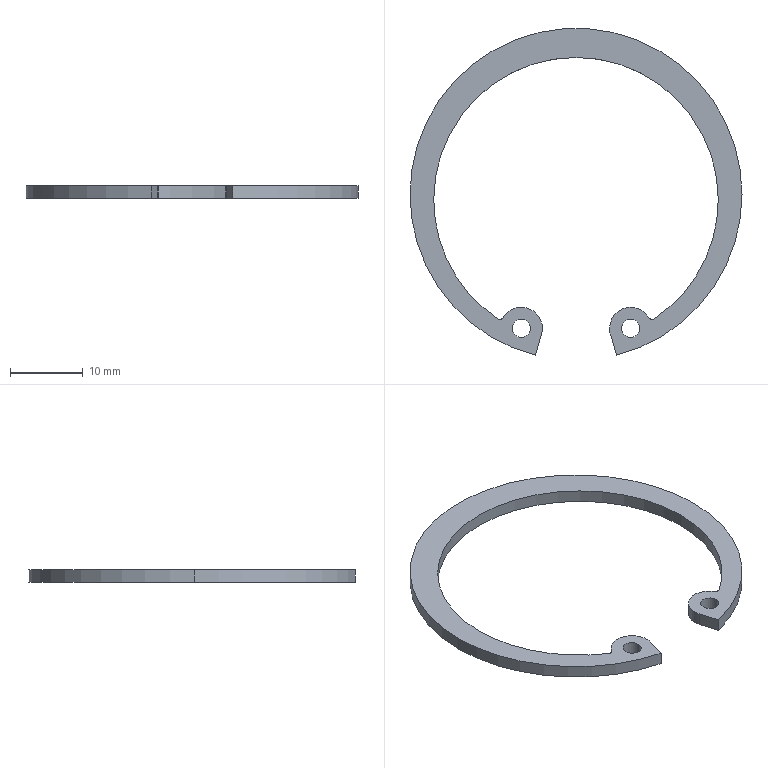Part | STEP file | BFU-2-42(2)^BFU71-6004ZZ-L55-S20_Drive roller assembly | 1 solid | 19 faces | box 45.5 x 44.807 x 1.75 mm | volume 744.242 mm3 | cylinder 15 | plane 4 | commonest cylinder face diameters 2.5 x4 5.8 x3 38.99 x3 45.5 x3 1 x2
STEP:
#1=CARTESIAN_POINT('',(0.,0.,0.));
#2=DIRECTION('',(0.,0.,1.));
#3=DIRECTION('',(1.,0.,0.));
#4=AXIS2_PLACEMENT_3D('',#1,#2,#3);
#5=CARTESIAN_POINT('',(22.75,0.005092,1.75));
#6=VERTEX_POINT('',#5);
#7=CARTESIAN_POINT('',(-22.75,0.005092,1.75));
#8=VERTEX_POINT('',#7);
#9=CARTESIAN_POINT('',(0.,0.005092,1.75));
#10=DIRECTION('',(0.,0.,1.));
#11=DIRECTION('',(1.,0.,0.));
#12=AXIS2_PLACEMENT_3D('',#9,#10,#11);
#13=CIRCLE('',#12,22.75);
#14=CARTESIAN_POINT('',(0.,0.005092,1.75));
#15=DIRECTION('',(0.,0.,-1.));
#16=DIRECTION('',(-1.,0.,0.));
#17=AXIS2_PLACEMENT_3D('',#14,#15,#16);
#18=CYLINDRICAL_SURFACE('',#17,22.75);
#19=CARTESIAN_POINT('',(3.142,0.));
#20=DIRECTION('',(-1.,0.));
#21=VECTOR('',#20,1.);
#22=LINE('',#19,#21);
#23=(GEOMETRIC_REPRESENTATION_CONTEXT(2)PARAMETRIC_REPRESENTATION_CONTEXT()REPRESENTATION_CONTEXT('',''));
#24=DEFINITIONAL_REPRESENTATION('',(#22),#23);
#25=PCURVE('',#18,#24);
#26=CARTESIAN_POINT('',(0.,0.005092,1.75));
#27=DIRECTION('',(0.,0.,1.));
#28=DIRECTION('',(1.,0.,0.));
#29=AXIS2_PLACEMENT_3D('',#26,#27,#28);
#30=PLANE('',#29);
#31=CARTESIAN_POINT('',(0.,0.));
#32=DIRECTION('',(1.,0.));
#33=AXIS2_PLACEMENT_2D('',#31,#32);
#34=CIRCLE('',#33,22.75);
#35=(GEOMETRIC_REPRESENTATION_CONTEXT(2)PARAMETRIC_REPRESENTATION_CONTEXT()REPRESENTATION_CONTEXT('',''));
#36=DEFINITIONAL_REPRESENTATION('',(#34),#35);
#37=PCURVE('',#30,#36);
#38=SURFACE_CURVE('',#13,(#25,#37),.PCURVE_S1.);
#39=EDGE_CURVE('',#6,#8,#38,.T.);
#40=ORIENTED_EDGE('',*,*,#39,.F.);
#41=CARTESIAN_POINT('',(22.75,0.005092,0.));
#42=VERTEX_POINT('',#41);
#43=CARTESIAN_POINT('',(22.75,0.005092,1.75));
#44=DIRECTION('',(0.,0.,-1.));
#45=VECTOR('',#44,1.);
#46=LINE('',#43,#45);
#47=CARTESIAN_POINT('',(3.142,0.));
#48=DIRECTION('',(0.,1.));
#49=VECTOR('',#48,1.);
#50=LINE('',#47,#49);
#51=(GEOMETRIC_REPRESENTATION_CONTEXT(2)PARAMETRIC_REPRESENTATION_CONTEXT()REPRESENTATION_CONTEXT('',''));
#52=DEFINITIONAL_REPRESENTATION('',(#50),#51);
#53=PCURVE('',#18,#52);
#54=CARTESIAN_POINT('',(0.,0.005092,1.75));
#55=DIRECTION('',(0.,0.,-1.));
#56=DIRECTION('',(-1.,0.,0.));
#57=AXIS2_PLACEMENT_3D('',#54,#55,#56);
#58=CYLINDRICAL_SURFACE('',#57,22.75);
#59=CARTESIAN_POINT('',(3.142,0.));
#60=DIRECTION('',(0.,1.));
#61=VECTOR('',#60,1.);
#62=LINE('',#59,#61);
#63=(GEOMETRIC_REPRESENTATION_CONTEXT(2)PARAMETRIC_REPRESENTATION_CONTEXT()REPRESENTATION_CONTEXT('',''));
#64=DEFINITIONAL_REPRESENTATION('',(#62),#63);
#65=PCURVE('',#58,#64);
#66=SURFACE_CURVE('',#46,(#53,#65),.PCURVE_S1.);
#67=EDGE_CURVE('',#6,#42,#66,.T.);
#68=ORIENTED_EDGE('',*,*,#67,.T.);
#69=CARTESIAN_POINT('',(-22.75,0.005092,0.));
#70=VERTEX_POINT('',#69);
#71=CARTESIAN_POINT('',(0.,0.005092,0.));
#72=DIRECTION('',(0.,0.,1.));
#73=DIRECTION('',(1.,0.,0.));
#74=AXIS2_PLACEMENT_3D('',#71,#72,#73);
#75=CIRCLE('',#74,22.75);
#76=CARTESIAN_POINT('',(3.142,1.75));
#77=DIRECTION('',(-1.,0.));
#78=VECTOR('',#77,1.);
#79=LINE('',#76,#78);
#80=(GEOMETRIC_REPRESENTATION_CONTEXT(2)PARAMETRIC_REPRESENTATION_CONTEXT()REPRESENTATION_CONTEXT('',''));
#81=DEFINITIONAL_REPRESENTATION('',(#79),#80);
#82=PCURVE('',#18,#81);
#83=CARTESIAN_POINT('',(0.,0.005092,0.));
#84=DIRECTION('',(0.,0.,1.));
#85=DIRECTION('',(1.,0.,0.));
#86=AXIS2_PLACEMENT_3D('',#83,#84,#85);
#87=PLANE('',#86);
#88=CARTESIAN_POINT('',(0.,0.));
#89=DIRECTION('',(1.,0.));
#90=AXIS2_PLACEMENT_2D('',#88,#89);
#91=CIRCLE('',#90,22.75);
#92=(GEOMETRIC_REPRESENTATION_CONTEXT(2)PARAMETRIC_REPRESENTATION_CONTEXT()REPRESENTATION_CONTEXT('',''));
#93=DEFINITIONAL_REPRESENTATION('',(#91),#92);
#94=PCURVE('',#87,#93);
#95=SURFACE_CURVE('',#75,(#82,#94),.PCURVE_S1.);
#96=EDGE_CURVE('',#42,#70,#95,.T.);
#97=ORIENTED_EDGE('',*,*,#96,.T.);
#98=CARTESIAN_POINT('',(-22.75,0.005092,1.75));
#99=DIRECTION('',(0.,0.,-1.));
#100=VECTOR('',#99,1.);
#101=LINE('',#98,#100);
#102=CARTESIAN_POINT('',(0.,0.));
#103=DIRECTION('',(0.,1.));
#104=VECTOR('',#103,1.);
#105=LINE('',#102,#104);
#106=(GEOMETRIC_REPRESENTATION_CONTEXT(2)PARAMETRIC_REPRESENTATION_CONTEXT()REPRESENTATION_CONTEXT('',''));
#107=DEFINITIONAL_REPRESENTATION('',(#105),#106);
#108=PCURVE('',#18,#107);
#109=CARTESIAN_POINT('',(0.,0.005092,1.75));
#110=DIRECTION('',(0.,0.,-1.));
#111=DIRECTION('',(-1.,0.,0.));
#112=AXIS2_PLACEMENT_3D('',#109,#110,#111);
#113=CYLINDRICAL_SURFACE('',#112,22.75);
#114=CARTESIAN_POINT('',(6.283,0.));
#115=DIRECTION('',(0.,1.));
#116=VECTOR('',#115,1.);
#117=LINE('',#114,#116);
#118=(GEOMETRIC_REPRESENTATION_CONTEXT(2)PARAMETRIC_REPRESENTATION_CONTEXT()REPRESENTATION_CONTEXT('',''));
#119=DEFINITIONAL_REPRESENTATION('',(#117),#118);
#120=PCURVE('',#113,#119);
#121=SURFACE_CURVE('',#101,(#108,#120),.PCURVE_S1.);
#122=EDGE_CURVE('',#8,#70,#121,.T.);
#123=ORIENTED_EDGE('',*,*,#122,.F.);
#124=EDGE_LOOP('',(#40,#68,#97,#123));
#125=FACE_BOUND('',#124,.T.);
#126=ADVANCED_FACE('',(#125),#18,.T.);
#127=CARTESIAN_POINT('',(-5.572,-22.052,1.75));
#128=VERTEX_POINT('',#127);
#129=CARTESIAN_POINT('',(0.,0.005092,1.75));
#130=DIRECTION('',(0.,0.,1.));
#131=DIRECTION('',(1.,0.,0.));
#132=AXIS2_PLACEMENT_3D('',#129,#130,#131);
#133=CIRCLE('',#132,22.75);
#134=CARTESIAN_POINT('',(9.425,0.));
#135=DIRECTION('',(-1.,0.));
#136=VECTOR('',#135,1.);
#137=LINE('',#134,#136);
#138=(GEOMETRIC_REPRESENTATION_CONTEXT(2)PARAMETRIC_REPRESENTATION_CONTEXT()REPRESENTATION_CONTEXT('',''));
#139=DEFINITIONAL_REPRESENTATION('',(#137),#138);
#140=PCURVE('',#113,#139);
#141=CARTESIAN_POINT('',(0.,0.));
#142=DIRECTION('',(1.,0.));
#143=AXIS2_PLACEMENT_2D('',#141,#142);
#144=CIRCLE('',#143,22.75);
#145=(GEOMETRIC_REPRESENTATION_CONTEXT(2)PARAMETRIC_REPRESENTATION_CONTEXT()REPRESENTATION_CONTEXT('',''));
#146=DEFINITIONAL_REPRESENTATION('',(#144),#145);
#147=PCURVE('',#30,#146);
#148=SURFACE_CURVE('',#133,(#140,#147),.PCURVE_S1.);
#149=EDGE_CURVE('',#8,#128,#148,.T.);
#150=ORIENTED_EDGE('',*,*,#149,.F.);
#151=ORIENTED_EDGE('',*,*,#122,.T.);
#152=CARTESIAN_POINT('',(-5.572,-22.052,0.));
#153=VERTEX_POINT('',#152);
#154=CARTESIAN_POINT('',(0.,0.005092,0.));
#155=DIRECTION('',(0.,0.,1.));
#156=DIRECTION('',(1.,0.,0.));
#157=AXIS2_PLACEMENT_3D('',#154,#155,#156);
#158=CIRCLE('',#157,22.75);
#159=CARTESIAN_POINT('',(9.425,1.75));
#160=DIRECTION('',(-1.,0.));
#161=VECTOR('',#160,1.);
#162=LINE('',#159,#161);
#163=(GEOMETRIC_REPRESENTATION_CONTEXT(2)PARAMETRIC_REPRESENTATION_CONTEXT()REPRESENTATION_CONTEXT('',''));
#164=DEFINITIONAL_REPRESENTATION('',(#162),#163);
#165=PCURVE('',#113,#164);
#166=CARTESIAN_POINT('',(0.,0.));
#167=DIRECTION('',(1.,0.));
#168=AXIS2_PLACEMENT_2D('',#166,#167);
#169=CIRCLE('',#168,22.75);
#170=(GEOMETRIC_REPRESENTATION_CONTEXT(2)PARAMETRIC_REPRESENTATION_CONTEXT()REPRESENTATION_CONTEXT('',''));
#171=DEFINITIONAL_REPRESENTATION('',(#169),#170);
#172=PCURVE('',#87,#171);
#173=SURFACE_CURVE('',#158,(#165,#172),.PCURVE_S1.);
#174=EDGE_CURVE('',#70,#153,#173,.T.);
#175=ORIENTED_EDGE('',*,*,#174,.T.);
#176=CARTESIAN_POINT('',(-5.572,-22.052,1.75));
#177=DIRECTION('',(0.,0.,-1.));
#178=VECTOR('',#177,1.);
#179=LINE('',#176,#178);
#180=CARTESIAN_POINT('',(4.96,0.));
#181=DIRECTION('',(0.,1.));
#182=VECTOR('',#181,1.);
#183=LINE('',#180,#182);
#184=(GEOMETRIC_REPRESENTATION_CONTEXT(2)PARAMETRIC_REPRESENTATION_CONTEXT()REPRESENTATION_CONTEXT('',''));
#185=DEFINITIONAL_REPRESENTATION('',(#183),#184);
#186=PCURVE('',#113,#185);
#187=CARTESIAN_POINT('',(-5.572,-22.052,1.75));
#188=DIRECTION('',(-0.9582,0.286,0.));
#189=DIRECTION('',(0.,0.,1.));
#190=AXIS2_PLACEMENT_3D('',#187,#188,#189);
#191=PLANE('',#190);
#192=CARTESIAN_POINT('',(0.,0.));
#193=DIRECTION('',(-1.,0.));
#194=VECTOR('',#193,1.);
#195=LINE('',#192,#194);
#196=(GEOMETRIC_REPRESENTATION_CONTEXT(2)PARAMETRIC_REPRESENTATION_CONTEXT()REPRESENTATION_CONTEXT('',''));
#197=DEFINITIONAL_REPRESENTATION('',(#195),#196);
#198=PCURVE('',#191,#197);
#199=SURFACE_CURVE('',#179,(#186,#198),.PCURVE_S1.);
#200=EDGE_CURVE('',#128,#153,#199,.T.);
#201=ORIENTED_EDGE('',*,*,#200,.F.);
#202=EDGE_LOOP('',(#150,#151,#175,#201));
#203=FACE_BOUND('',#202,.T.);
#204=ADVANCED_FACE('',(#203),#113,.T.);
#205=CARTESIAN_POINT('',(10.69,-17.044,1.75));
#206=VERTEX_POINT('',#205);
#207=CARTESIAN_POINT('',(10.69,-17.044,0.));
#208=VERTEX_POINT('',#207);
#209=CARTESIAN_POINT('',(10.69,-17.044,1.75));
#210=DIRECTION('',(0.,0.,-1.));
#211=VECTOR('',#210,1.);
#212=LINE('',#209,#211);
#213=CARTESIAN_POINT('',(-0.0005,-0.7416,1.75));
#214=DIRECTION('',(0.,0.,-1.));
#215=DIRECTION('',(-1.,0.,0.));
#216=AXIS2_PLACEMENT_3D('',#213,#214,#215);
#217=CYLINDRICAL_SURFACE('',#216,19.495);
#218=CARTESIAN_POINT('',(4.132,0.));
#219=DIRECTION('',(0.,1.));
#220=VECTOR('',#219,1.);
#221=LINE('',#218,#220);
#222=(GEOMETRIC_REPRESENTATION_CONTEXT(2)PARAMETRIC_REPRESENTATION_CONTEXT()REPRESENTATION_CONTEXT('',''));
#223=DEFINITIONAL_REPRESENTATION('',(#221),#222);
#224=PCURVE('',#217,#223);
#225=CARTESIAN_POINT('',(10.416,-16.626,1.75));
#226=DIRECTION('',(0.,0.,-1.));
#227=DIRECTION('',(-1.,0.,0.));
#228=AXIS2_PLACEMENT_3D('',#225,#226,#227);
#229=CYLINDRICAL_SURFACE('',#228,0.5);
#230=CARTESIAN_POINT('',(4.132,0.));
#231=DIRECTION('',(0.,1.));
#232=VECTOR('',#231,1.);
#233=LINE('',#230,#232);
#234=(GEOMETRIC_REPRESENTATION_CONTEXT(2)PARAMETRIC_REPRESENTATION_CONTEXT()REPRESENTATION_CONTEXT('',''));
#235=DEFINITIONAL_REPRESENTATION('',(#233),#234);
#236=PCURVE('',#229,#235);
#237=SURFACE_CURVE('',#212,(#224,#236),.PCURVE_S1.);
#238=EDGE_CURVE('',#206,#208,#237,.T.);
#239=ORIENTED_EDGE('',*,*,#238,.T.);
#240=CARTESIAN_POINT('',(19.494,-0.7416,0.));
#241=VERTEX_POINT('',#240);
#242=CARTESIAN_POINT('',(-0.0005,-0.7416,0.));
#243=DIRECTION('',(0.,0.,1.));
#244=DIRECTION('',(1.,0.,0.));
#245=AXIS2_PLACEMENT_3D('',#242,#243,#244);
#246=CIRCLE('',#245,19.495);
#247=CARTESIAN_POINT('',(9.425,1.75));
#248=DIRECTION('',(-1.,0.));
#249=VECTOR('',#248,1.);
#250=LINE('',#247,#249);
#251=(GEOMETRIC_REPRESENTATION_CONTEXT(2)PARAMETRIC_REPRESENTATION_CONTEXT()REPRESENTATION_CONTEXT('',''));
#252=DEFINITIONAL_REPRESENTATION('',(#250),#251);
#253=PCURVE('',#217,#252);
#254=CARTESIAN_POINT('',(-0.0005,-0.7467));
#255=DIRECTION('',(1.,0.));
#256=AXIS2_PLACEMENT_2D('',#254,#255);
#257=CIRCLE('',#256,19.495);
#258=(GEOMETRIC_REPRESENTATION_CONTEXT(2)PARAMETRIC_REPRESENTATION_CONTEXT()REPRESENTATION_CONTEXT('',''));
#259=DEFINITIONAL_REPRESENTATION('',(#257),#258);
#260=PCURVE('',#87,#259);
#261=SURFACE_CURVE('',#246,(#253,#260),.PCURVE_S1.);
#262=EDGE_CURVE('',#208,#241,#261,.T.);
#263=ORIENTED_EDGE('',*,*,#262,.T.);
#264=CARTESIAN_POINT('',(19.494,-0.7416,1.75));
#265=VERTEX_POINT('',#264);
#266=CARTESIAN_POINT('',(19.494,-0.7416,1.75));
#267=DIRECTION('',(0.,0.,-1.));
#268=VECTOR('',#267,1.);
#269=LINE('',#266,#268);
#270=CARTESIAN_POINT('',(3.142,0.));
#271=DIRECTION('',(0.,1.));
#272=VECTOR('',#271,1.);
#273=LINE('',#270,#272);
#274=(GEOMETRIC_REPRESENTATION_CONTEXT(2)PARAMETRIC_REPRESENTATION_CONTEXT()REPRESENTATION_CONTEXT('',''));
#275=DEFINITIONAL_REPRESENTATION('',(#273),#274);
#276=PCURVE('',#217,#275);
#277=CARTESIAN_POINT('',(-0.0005,-0.7416,1.75));
#278=DIRECTION('',(0.,0.,-1.));
#279=DIRECTION('',(-1.,0.,0.));
#280=AXIS2_PLACEMENT_3D('',#277,#278,#279);
#281=CYLINDRICAL_SURFACE('',#280,19.495);
#282=CARTESIAN_POINT('',(3.142,0.));
#283=DIRECTION('',(0.,1.));
#284=VECTOR('',#283,1.);
#285=LINE('',#282,#284);
#286=(GEOMETRIC_REPRESENTATION_CONTEXT(2)PARAMETRIC_REPRESENTATION_CONTEXT()REPRESENTATION_CONTEXT('',''));
#287=DEFINITIONAL_REPRESENTATION('',(#285),#286);
#288=PCURVE('',#281,#287);
#289=SURFACE_CURVE('',#269,(#276,#288),.PCURVE_S1.);
#290=EDGE_CURVE('',#265,#241,#289,.T.);
#291=ORIENTED_EDGE('',*,*,#290,.F.);
#292=CARTESIAN_POINT('',(-0.0005,-0.7416,1.75));
#293=DIRECTION('',(0.,0.,1.));
#294=DIRECTION('',(1.,0.,0.));
#295=AXIS2_PLACEMENT_3D('',#292,#293,#294);
#296=CIRCLE('',#295,19.495);
#297=CARTESIAN_POINT('',(9.425,0.));
#298=DIRECTION('',(-1.,0.));
#299=VECTOR('',#298,1.);
#300=LINE('',#297,#299);
#301=(GEOMETRIC_REPRESENTATION_CONTEXT(2)PARAMETRIC_REPRESENTATION_CONTEXT()REPRESENTATION_CONTEXT('',''));
#302=DEFINITIONAL_REPRESENTATION('',(#300),#301);
#303=PCURVE('',#217,#302);
#304=CARTESIAN_POINT('',(-0.0005,-0.7467));
#305=DIRECTION('',(1.,0.));
#306=AXIS2_PLACEMENT_2D('',#304,#305);
#307=CIRCLE('',#306,19.495);
#308=(GEOMETRIC_REPRESENTATION_CONTEXT(2)PARAMETRIC_REPRESENTATION_CONTEXT()REPRESENTATION_CONTEXT('',''));
#309=DEFINITIONAL_REPRESENTATION('',(#307),#308);
#310=PCURVE('',#30,#309);
#311=SURFACE_CURVE('',#296,(#303,#310),.PCURVE_S1.);
#312=EDGE_CURVE('',#206,#265,#311,.T.);
#313=ORIENTED_EDGE('',*,*,#312,.F.);
#314=EDGE_LOOP('',(#239,#263,#291,#313));
#315=FACE_BOUND('',#314,.F.);
#316=ADVANCED_FACE('',(#315),#217,.F.);
#317=CARTESIAN_POINT('',(-19.495,-0.7416,0.));
#318=VERTEX_POINT('',#317);
#319=CARTESIAN_POINT('',(-0.0005,-0.7416,0.));
#320=DIRECTION('',(0.,0.,1.));
#321=DIRECTION('',(1.,0.,0.));
#322=AXIS2_PLACEMENT_3D('',#319,#320,#321);
#323=CIRCLE('',#322,19.495);
#324=CARTESIAN_POINT('',(3.142,1.75));
#325=DIRECTION('',(-1.,0.));
#326=VECTOR('',#325,1.);
#327=LINE('',#324,#326);
#328=(GEOMETRIC_REPRESENTATION_CONTEXT(2)PARAMETRIC_REPRESENTATION_CONTEXT()REPRESENTATION_CONTEXT('',''));
#329=DEFINITIONAL_REPRESENTATION('',(#327),#328);
#330=PCURVE('',#281,#329);
#331=CARTESIAN_POINT('',(-0.0005,-0.7467));
#332=DIRECTION('',(1.,0.));
#333=AXIS2_PLACEMENT_2D('',#331,#332);
#334=CIRCLE('',#333,19.495);
#335=(GEOMETRIC_REPRESENTATION_CONTEXT(2)PARAMETRIC_REPRESENTATION_CONTEXT()REPRESENTATION_CONTEXT('',''));
#336=DEFINITIONAL_REPRESENTATION('',(#334),#335);
#337=PCURVE('',#87,#336);
#338=SURFACE_CURVE('',#323,(#330,#337),.PCURVE_S1.);
#339=EDGE_CURVE('',#241,#318,#338,.T.);
#340=ORIENTED_EDGE('',*,*,#339,.T.);
#341=CARTESIAN_POINT('',(-19.495,-0.7416,1.75));
#342=VERTEX_POINT('',#341);
#343=CARTESIAN_POINT('',(-19.495,-0.7416,1.75));
#344=DIRECTION('',(0.,0.,-1.));
#345=VECTOR('',#344,1.);
#346=LINE('',#343,#345);
#347=CARTESIAN_POINT('',(0.,0.));
#348=DIRECTION('',(0.,1.));
#349=VECTOR('',#348,1.);
#350=LINE('',#347,#349);
#351=(GEOMETRIC_REPRESENTATION_CONTEXT(2)PARAMETRIC_REPRESENTATION_CONTEXT()REPRESENTATION_CONTEXT('',''));
#352=DEFINITIONAL_REPRESENTATION('',(#350),#351);
#353=PCURVE('',#281,#352);
#354=CARTESIAN_POINT('',(-0.0005,-0.7416,1.75));
#355=DIRECTION('',(0.,0.,-1.));
#356=DIRECTION('',(-1.,0.,0.));
#357=AXIS2_PLACEMENT_3D('',#354,#355,#356);
#358=CYLINDRICAL_SURFACE('',#357,19.495);
#359=CARTESIAN_POINT('',(6.283,0.));
#360=DIRECTION('',(0.,1.));
#361=VECTOR('',#360,1.);
#362=LINE('',#359,#361);
#363=(GEOMETRIC_REPRESENTATION_CONTEXT(2)PARAMETRIC_REPRESENTATION_CONTEXT()REPRESENTATION_CONTEXT('',''));
#364=DEFINITIONAL_REPRESENTATION('',(#362),#363);
#365=PCURVE('',#358,#364);
#366=SURFACE_CURVE('',#346,(#353,#365),.PCURVE_S1.);
#367=EDGE_CURVE('',#342,#318,#366,.T.);
#368=ORIENTED_EDGE('',*,*,#367,.F.);
#369=CARTESIAN_POINT('',(-0.0005,-0.7416,1.75));
#370=DIRECTION('',(0.,0.,1.));
#371=DIRECTION('',(1.,0.,0.));
#372=AXIS2_PLACEMENT_3D('',#369,#370,#371);
#373=CIRCLE('',#372,19.495);
#374=CARTESIAN_POINT('',(3.142,0.));
#375=DIRECTION('',(-1.,0.));
#376=VECTOR('',#375,1.);
#377=LINE('',#374,#376);
#378=(GEOMETRIC_REPRESENTATION_CONTEXT(2)PARAMETRIC_REPRESENTATION_CONTEXT()REPRESENTATION_CONTEXT('',''));
#379=DEFINITIONAL_REPRESENTATION('',(#377),#378);
#380=PCURVE('',#281,#379);
#381=CARTESIAN_POINT('',(-0.0005,-0.7467));
#382=DIRECTION('',(1.,0.));
#383=AXIS2_PLACEMENT_2D('',#381,#382);
#384=CIRCLE('',#383,19.495);
#385=(GEOMETRIC_REPRESENTATION_CONTEXT(2)PARAMETRIC_REPRESENTATION_CONTEXT()REPRESENTATION_CONTEXT('',''));
#386=DEFINITIONAL_REPRESENTATION('',(#384),#385);
#387=PCURVE('',#30,#386);
#388=SURFACE_CURVE('',#373,(#380,#387),.PCURVE_S1.);
#389=EDGE_CURVE('',#265,#342,#388,.T.);
#390=ORIENTED_EDGE('',*,*,#389,.F.);
#391=ORIENTED_EDGE('',*,*,#290,.T.);
#392=EDGE_LOOP('',(#340,#368,#390,#391));
#393=FACE_BOUND('',#392,.F.);
#394=ADVANCED_FACE('',(#393),#281,.F.);
#395=CARTESIAN_POINT('',(6.25,-18.374,1.75));
#396=VERTEX_POINT('',#395);
#397=CARTESIAN_POINT('',(6.25,-18.374,0.));
#398=VERTEX_POINT('',#397);
#399=CARTESIAN_POINT('',(6.25,-18.374,1.75));
#400=DIRECTION('',(0.,0.,-1.));
#401=VECTOR('',#400,1.);
#402=LINE('',#399,#401);
#403=CARTESIAN_POINT('',(7.5,-18.374,1.75));
#404=DIRECTION('',(0.,0.,-1.));
#405=DIRECTION('',(-1.,0.,0.));
#406=AXIS2_PLACEMENT_3D('',#403,#404,#405);
#407=CYLINDRICAL_SURFACE('',#406,1.25);
#408=CARTESIAN_POINT('',(6.283,0.));
#409=DIRECTION('',(0.,1.));
#410=VECTOR('',#409,1.);
#411=LINE('',#408,#410);
#412=(GEOMETRIC_REPRESENTATION_CONTEXT(2)PARAMETRIC_REPRESENTATION_CONTEXT()REPRESENTATION_CONTEXT('',''));
#413=DEFINITIONAL_REPRESENTATION('',(#411),#412);
#414=PCURVE('',#407,#413);
#415=CARTESIAN_POINT('',(7.5,-18.374,1.75));
#416=DIRECTION('',(0.,0.,-1.));
#417=DIRECTION('',(-1.,0.,0.));
#418=AXIS2_PLACEMENT_3D('',#415,#416,#417);
#419=CYLINDRICAL_SURFACE('',#418,1.25);
#420=CARTESIAN_POINT('',(0.,0.));
#421=DIRECTION('',(0.,1.));
#422=VECTOR('',#421,1.);
#423=LINE('',#420,#422);
#424=(GEOMETRIC_REPRESENTATION_CONTEXT(2)PARAMETRIC_REPRESENTATION_CONTEXT()REPRESENTATION_CONTEXT('',''));
#425=DEFINITIONAL_REPRESENTATION('',(#423),#424);
#426=PCURVE('',#419,#425);
#427=SURFACE_CURVE('',#402,(#414,#426),.PCURVE_S1.);
#428=EDGE_CURVE('',#396,#398,#427,.T.);
#429=ORIENTED_EDGE('',*,*,#428,.T.);
#430=CARTESIAN_POINT('',(8.75,-18.374,0.));
#431=VERTEX_POINT('',#430);
#432=CARTESIAN_POINT('',(7.5,-18.374,0.));
#433=DIRECTION('',(0.,0.,1.));
#434=DIRECTION('',(1.,0.,0.));
#435=AXIS2_PLACEMENT_3D('',#432,#433,#434);
#436=CIRCLE('',#435,1.25);
#437=CARTESIAN_POINT('',(9.425,1.75));
#438=DIRECTION('',(-1.,0.));
#439=VECTOR('',#438,1.);
#440=LINE('',#437,#439);
#441=(GEOMETRIC_REPRESENTATION_CONTEXT(2)PARAMETRIC_REPRESENTATION_CONTEXT()REPRESENTATION_CONTEXT('',''));
#442=DEFINITIONAL_REPRESENTATION('',(#440),#441);
#443=PCURVE('',#407,#442);
#444=CARTESIAN_POINT('',(7.5,-18.379));
#445=DIRECTION('',(1.,0.));
#446=AXIS2_PLACEMENT_2D('',#444,#445);
#447=CIRCLE('',#446,1.25);
#448=(GEOMETRIC_REPRESENTATION_CONTEXT(2)PARAMETRIC_REPRESENTATION_CONTEXT()REPRESENTATION_CONTEXT('',''));
#449=DEFINITIONAL_REPRESENTATION('',(#447),#448);
#450=PCURVE('',#87,#449);
#451=SURFACE_CURVE('',#436,(#443,#450),.PCURVE_S1.);
#452=EDGE_CURVE('',#398,#431,#451,.T.);
#453=ORIENTED_EDGE('',*,*,#452,.T.);
#454=CARTESIAN_POINT('',(8.75,-18.374,1.75));
#455=VERTEX_POINT('',#454);
#456=CARTESIAN_POINT('',(8.75,-18.374,1.75));
#457=DIRECTION('',(0.,0.,-1.));
#458=VECTOR('',#457,1.);
#459=LINE('',#456,#458);
#460=CARTESIAN_POINT('',(3.142,0.));
#461=DIRECTION('',(0.,1.));
#462=VECTOR('',#461,1.);
#463=LINE('',#460,#462);
#464=(GEOMETRIC_REPRESENTATION_CONTEXT(2)PARAMETRIC_REPRESENTATION_CONTEXT()REPRESENTATION_CONTEXT('',''));
#465=DEFINITIONAL_REPRESENTATION('',(#463),#464);
#466=PCURVE('',#407,#465);
#467=CARTESIAN_POINT('',(3.142,0.));
#468=DIRECTION('',(0.,1.));
#469=VECTOR('',#468,1.);
#470=LINE('',#467,#469);
#471=(GEOMETRIC_REPRESENTATION_CONTEXT(2)PARAMETRIC_REPRESENTATION_CONTEXT()REPRESENTATION_CONTEXT('',''));
#472=DEFINITIONAL_REPRESENTATION('',(#470),#471);
#473=PCURVE('',#419,#472);
#474=SURFACE_CURVE('',#459,(#466,#473),.PCURVE_S1.);
#475=EDGE_CURVE('',#455,#431,#474,.T.);
#476=ORIENTED_EDGE('',*,*,#475,.F.);
#477=CARTESIAN_POINT('',(7.5,-18.374,1.75));
#478=DIRECTION('',(0.,0.,1.));
#479=DIRECTION('',(1.,0.,0.));
#480=AXIS2_PLACEMENT_3D('',#477,#478,#479);
#481=CIRCLE('',#480,1.25);
#482=CARTESIAN_POINT('',(9.425,0.));
#483=DIRECTION('',(-1.,0.));
#484=VECTOR('',#483,1.);
#485=LINE('',#482,#484);
#486=(GEOMETRIC_REPRESENTATION_CONTEXT(2)PARAMETRIC_REPRESENTATION_CONTEXT()REPRESENTATION_CONTEXT('',''));
#487=DEFINITIONAL_REPRESENTATION('',(#485),#486);
#488=PCURVE('',#407,#487);
#489=CARTESIAN_POINT('',(7.5,-18.379));
#490=DIRECTION('',(1.,0.));
#491=AXIS2_PLACEMENT_2D('',#489,#490);
#492=CIRCLE('',#491,1.25);
#493=(GEOMETRIC_REPRESENTATION_CONTEXT(2)PARAMETRIC_REPRESENTATION_CONTEXT()REPRESENTATION_CONTEXT('',''));
#494=DEFINITIONAL_REPRESENTATION('',(#492),#493);
#495=PCURVE('',#30,#494);
#496=SURFACE_CURVE('',#481,(#488,#495),.PCURVE_S1.);
#497=EDGE_CURVE('',#396,#455,#496,.T.);
#498=ORIENTED_EDGE('',*,*,#497,.F.);
#499=EDGE_LOOP('',(#429,#453,#476,#498));
#500=FACE_BOUND('',#499,.F.);
#501=ADVANCED_FACE('',(#500),#407,.F.);
#502=CARTESIAN_POINT('',(-8.75,-18.374,1.75));
#503=VERTEX_POINT('',#502);
#504=CARTESIAN_POINT('',(-8.75,-18.374,0.));
#505=VERTEX_POINT('',#504);
#506=CARTESIAN_POINT('',(-8.75,-18.374,1.75));
#507=DIRECTION('',(0.,0.,-1.));
#508=VECTOR('',#507,1.);
#509=LINE('',#506,#508);
#510=CARTESIAN_POINT('',(-7.5,-18.374,1.75));
#511=DIRECTION('',(0.,0.,-1.));
#512=DIRECTION('',(-1.,0.,0.));
#513=AXIS2_PLACEMENT_3D('',#510,#511,#512);
#514=CYLINDRICAL_SURFACE('',#513,1.25);
#515=CARTESIAN_POINT('',(6.283,0.));
#516=DIRECTION('',(0.,1.));
#517=VECTOR('',#516,1.);
#518=LINE('',#515,#517);
#519=(GEOMETRIC_REPRESENTATION_CONTEXT(2)PARAMETRIC_REPRESENTATION_CONTEXT()REPRESENTATION_CONTEXT('',''));
#520=DEFINITIONAL_REPRESENTATION('',(#518),#519);
#521=PCURVE('',#514,#520);
#522=CARTESIAN_POINT('',(-7.5,-18.374,1.75));
#523=DIRECTION('',(0.,0.,-1.));
#524=DIRECTION('',(-1.,0.,0.));
#525=AXIS2_PLACEMENT_3D('',#522,#523,#524);
#526=CYLINDRICAL_SURFACE('',#525,1.25);
#527=CARTESIAN_POINT('',(0.,0.));
#528=DIRECTION('',(0.,1.));
#529=VECTOR('',#528,1.);
#530=LINE('',#527,#529);
#531=(GEOMETRIC_REPRESENTATION_CONTEXT(2)PARAMETRIC_REPRESENTATION_CONTEXT()REPRESENTATION_CONTEXT('',''));
#532=DEFINITIONAL_REPRESENTATION('',(#530),#531);
#533=PCURVE('',#526,#532);
#534=SURFACE_CURVE('',#509,(#521,#533),.PCURVE_S1.);
#535=EDGE_CURVE('',#503,#505,#534,.T.);
#536=ORIENTED_EDGE('',*,*,#535,.T.);
#537=CARTESIAN_POINT('',(-6.25,-18.374,0.));
#538=VERTEX_POINT('',#537);
#539=CARTESIAN_POINT('',(-7.5,-18.374,0.));
#540=DIRECTION('',(0.,0.,1.));
#541=DIRECTION('',(1.,0.,0.));
#542=AXIS2_PLACEMENT_3D('',#539,#540,#541);
#543=CIRCLE('',#542,1.25);
#544=CARTESIAN_POINT('',(9.425,1.75));
#545=DIRECTION('',(-1.,0.));
#546=VECTOR('',#545,1.);
#547=LINE('',#544,#546);
#548=(GEOMETRIC_REPRESENTATION_CONTEXT(2)PARAMETRIC_REPRESENTATION_CONTEXT()REPRESENTATION_CONTEXT('',''));
#549=DEFINITIONAL_REPRESENTATION('',(#547),#548);
#550=PCURVE('',#514,#549);
#551=CARTESIAN_POINT('',(-7.5,-18.379));
#552=DIRECTION('',(1.,0.));
#553=AXIS2_PLACEMENT_2D('',#551,#552);
#554=CIRCLE('',#553,1.25);
#555=(GEOMETRIC_REPRESENTATION_CONTEXT(2)PARAMETRIC_REPRESENTATION_CONTEXT()REPRESENTATION_CONTEXT('',''));
#556=DEFINITIONAL_REPRESENTATION('',(#554),#555);
#557=PCURVE('',#87,#556);
#558=SURFACE_CURVE('',#543,(#550,#557),.PCURVE_S1.);
#559=EDGE_CURVE('',#505,#538,#558,.T.);
#560=ORIENTED_EDGE('',*,*,#559,.T.);
#561=CARTESIAN_POINT('',(-6.25,-18.374,1.75));
#562=VERTEX_POINT('',#561);
#563=CARTESIAN_POINT('',(-6.25,-18.374,1.75));
#564=DIRECTION('',(0.,0.,-1.));
#565=VECTOR('',#564,1.);
#566=LINE('',#563,#565);
#567=CARTESIAN_POINT('',(3.142,0.));
#568=DIRECTION('',(0.,1.));
#569=VECTOR('',#568,1.);
#570=LINE('',#567,#569);
#571=(GEOMETRIC_REPRESENTATION_CONTEXT(2)PARAMETRIC_REPRESENTATION_CONTEXT()REPRESENTATION_CONTEXT('',''));
#572=DEFINITIONAL_REPRESENTATION('',(#570),#571);
#573=PCURVE('',#514,#572);
#574=CARTESIAN_POINT('',(3.142,0.));
#575=DIRECTION('',(0.,1.));
#576=VECTOR('',#575,1.);
#577=LINE('',#574,#576);
#578=(GEOMETRIC_REPRESENTATION_CONTEXT(2)PARAMETRIC_REPRESENTATION_CONTEXT()REPRESENTATION_CONTEXT('',''));
#579=DEFINITIONAL_REPRESENTATION('',(#577),#578);
#580=PCURVE('',#526,#579);
#581=SURFACE_CURVE('',#566,(#573,#580),.PCURVE_S1.);
#582=EDGE_CURVE('',#562,#538,#581,.T.);
#583=ORIENTED_EDGE('',*,*,#582,.F.);
#584=CARTESIAN_POINT('',(-7.5,-18.374,1.75));
#585=DIRECTION('',(0.,0.,1.));
#586=DIRECTION('',(1.,0.,0.));
#587=AXIS2_PLACEMENT_3D('',#584,#585,#586);
#588=CIRCLE('',#587,1.25);
#589=CARTESIAN_POINT('',(9.425,0.));
#590=DIRECTION('',(-1.,0.));
#591=VECTOR('',#590,1.);
#592=LINE('',#589,#591);
#593=(GEOMETRIC_REPRESENTATION_CONTEXT(2)PARAMETRIC_REPRESENTATION_CONTEXT()REPRESENTATION_CONTEXT('',''));
#594=DEFINITIONAL_REPRESENTATION('',(#592),#593);
#595=PCURVE('',#514,#594);
#596=CARTESIAN_POINT('',(-7.5,-18.379));
#597=DIRECTION('',(1.,0.));
#598=AXIS2_PLACEMENT_2D('',#596,#597);
#599=CIRCLE('',#598,1.25);
#600=(GEOMETRIC_REPRESENTATION_CONTEXT(2)PARAMETRIC_REPRESENTATION_CONTEXT()REPRESENTATION_CONTEXT('',''));
#601=DEFINITIONAL_REPRESENTATION('',(#599),#600);
#602=PCURVE('',#30,#601);
#603=SURFACE_CURVE('',#588,(#595,#602),.PCURVE_S1.);
#604=EDGE_CURVE('',#503,#562,#603,.T.);
#605=ORIENTED_EDGE('',*,*,#604,.F.);
#606=EDGE_LOOP('',(#536,#560,#583,#605));
#607=FACE_BOUND('',#606,.F.);
#608=ADVANCED_FACE('',(#607),#514,.F.);
#609=CARTESIAN_POINT('',(4.6,-18.374,1.75));
#610=VERTEX_POINT('',#609);
#611=CARTESIAN_POINT('',(4.721,-19.204,1.75));
#612=VERTEX_POINT('',#611);
#613=CARTESIAN_POINT('',(7.5,-18.374,1.75));
#614=DIRECTION('',(0.,0.,1.));
#615=DIRECTION('',(1.,0.,0.));
#616=AXIS2_PLACEMENT_3D('',#613,#614,#615);
#617=CIRCLE('',#616,2.9);
#618=CARTESIAN_POINT('',(7.5,-18.374,1.75));
#619=DIRECTION('',(0.,0.,-1.));
#620=DIRECTION('',(-1.,0.,0.));
#621=AXIS2_PLACEMENT_3D('',#618,#619,#620);
#622=CYLINDRICAL_SURFACE('',#621,2.9);
#623=CARTESIAN_POINT('',(9.425,0.));
#624=DIRECTION('',(-1.,0.));
#625=VECTOR('',#624,1.);
#626=LINE('',#623,#625);
#627=(GEOMETRIC_REPRESENTATION_CONTEXT(2)PARAMETRIC_REPRESENTATION_CONTEXT()REPRESENTATION_CONTEXT('',''));
#628=DEFINITIONAL_REPRESENTATION('',(#626),#627);
#629=PCURVE('',#622,#628);
#630=CARTESIAN_POINT('',(7.5,-18.379));
#631=DIRECTION('',(1.,0.));
#632=AXIS2_PLACEMENT_2D('',#630,#631);
#633=CIRCLE('',#632,2.9);
#634=(GEOMETRIC_REPRESENTATION_CONTEXT(2)PARAMETRIC_REPRESENTATION_CONTEXT()REPRESENTATION_CONTEXT('',''));
#635=DEFINITIONAL_REPRESENTATION('',(#633),#634);
#636=PCURVE('',#30,#635);
#637=SURFACE_CURVE('',#617,(#629,#636),.PCURVE_S1.);
#638=EDGE_CURVE('',#610,#612,#637,.T.);
#639=ORIENTED_EDGE('',*,*,#638,.F.);
#640=CARTESIAN_POINT('',(4.6,-18.374,0.));
#641=VERTEX_POINT('',#640);
#642=CARTESIAN_POINT('',(4.6,-18.374,1.75));
#643=DIRECTION('',(0.,0.,-1.));
#644=VECTOR('',#643,1.);
#645=LINE('',#642,#644);
#646=CARTESIAN_POINT('',(6.283,0.));
#647=DIRECTION('',(0.,1.));
#648=VECTOR('',#647,1.);
#649=LINE('',#646,#648);
#650=(GEOMETRIC_REPRESENTATION_CONTEXT(2)PARAMETRIC_REPRESENTATION_CONTEXT()REPRESENTATION_CONTEXT('',''));
#651=DEFINITIONAL_REPRESENTATION('',(#649),#650);
#652=PCURVE('',#622,#651);
#653=CARTESIAN_POINT('',(7.5,-18.374,1.75));
#654=DIRECTION('',(0.,0.,-1.));
#655=DIRECTION('',(-1.,0.,0.));
#656=AXIS2_PLACEMENT_3D('',#653,#654,#655);
#657=CYLINDRICAL_SURFACE('',#656,2.9);
#658=CARTESIAN_POINT('',(0.,0.));
#659=DIRECTION('',(0.,1.));
#660=VECTOR('',#659,1.);
#661=LINE('',#658,#660);
#662=(GEOMETRIC_REPRESENTATION_CONTEXT(2)PARAMETRIC_REPRESENTATION_CONTEXT()REPRESENTATION_CONTEXT('',''));
#663=DEFINITIONAL_REPRESENTATION('',(#661),#662);
#664=PCURVE('',#657,#663);
#665=SURFACE_CURVE('',#645,(#652,#664),.PCURVE_S1.);
#666=EDGE_CURVE('',#610,#641,#665,.T.);
#667=ORIENTED_EDGE('',*,*,#666,.T.);
#668=CARTESIAN_POINT('',(4.721,-19.204,0.));
#669=VERTEX_POINT('',#668);
#670=CARTESIAN_POINT('',(7.5,-18.374,0.));
#671=DIRECTION('',(0.,0.,1.));
#672=DIRECTION('',(1.,0.,0.));
#673=AXIS2_PLACEMENT_3D('',#670,#671,#672);
#674=CIRCLE('',#673,2.9);
#675=CARTESIAN_POINT('',(9.425,1.75));
#676=DIRECTION('',(-1.,0.));
#677=VECTOR('',#676,1.);
#678=LINE('',#675,#677);
#679=(GEOMETRIC_REPRESENTATION_CONTEXT(2)PARAMETRIC_REPRESENTATION_CONTEXT()REPRESENTATION_CONTEXT('',''));
#680=DEFINITIONAL_REPRESENTATION('',(#678),#679);
#681=PCURVE('',#622,#680);
#682=CARTESIAN_POINT('',(7.5,-18.379));
#683=DIRECTION('',(1.,0.));
#684=AXIS2_PLACEMENT_2D('',#682,#683);
#685=CIRCLE('',#684,2.9);
#686=(GEOMETRIC_REPRESENTATION_CONTEXT(2)PARAMETRIC_REPRESENTATION_CONTEXT()REPRESENTATION_CONTEXT('',''));
#687=DEFINITIONAL_REPRESENTATION('',(#685),#686);
#688=PCURVE('',#87,#687);
#689=SURFACE_CURVE('',#674,(#681,#688),.PCURVE_S1.);
#690=EDGE_CURVE('',#641,#669,#689,.T.);
#691=ORIENTED_EDGE('',*,*,#690,.T.);
#692=CARTESIAN_POINT('',(4.721,-19.204,1.75));
#693=DIRECTION('',(0.,0.,-1.));
#694=VECTOR('',#693,1.);
#695=LINE('',#692,#694);
#696=CARTESIAN_POINT('',(5.993,0.));
#697=DIRECTION('',(0.,1.));
#698=VECTOR('',#697,1.);
#699=LINE('',#696,#698);
#700=(GEOMETRIC_REPRESENTATION_CONTEXT(2)PARAMETRIC_REPRESENTATION_CONTEXT()REPRESENTATION_CONTEXT('',''));
#701=DEFINITIONAL_REPRESENTATION('',(#699),#700);
#702=PCURVE('',#622,#701);
#703=CARTESIAN_POINT('',(4.721,-19.204,1.75));
#704=DIRECTION('',(0.9581,0.2863,0.));
#705=DIRECTION('',(0.,0.,-1.));
#706=AXIS2_PLACEMENT_3D('',#703,#704,#705);
#707=PLANE('',#706);
#708=CARTESIAN_POINT('',(0.,0.));
#709=DIRECTION('',(1.,0.));
#710=VECTOR('',#709,1.);
#711=LINE('',#708,#710);
#712=(GEOMETRIC_REPRESENTATION_CONTEXT(2)PARAMETRIC_REPRESENTATION_CONTEXT()REPRESENTATION_CONTEXT('',''));
#713=DEFINITIONAL_REPRESENTATION('',(#711),#712);
#714=PCURVE('',#707,#713);
#715=SURFACE_CURVE('',#695,(#702,#714),.PCURVE_S1.);
#716=EDGE_CURVE('',#612,#669,#715,.T.);
#717=ORIENTED_EDGE('',*,*,#716,.F.);
#718=EDGE_LOOP('',(#639,#667,#691,#717));
#719=FACE_BOUND('',#718,.T.);
#720=ADVANCED_FACE('',(#719),#622,.T.);
#721=CARTESIAN_POINT('',(5.572,-22.052,0.));
#722=VERTEX_POINT('',#721);
#723=CARTESIAN_POINT('',(4.721,-19.204,0.));
#724=DIRECTION('',(0.2863,-0.9581,0.));
#725=VECTOR('',#724,1.);
#726=LINE('',#723,#725);
#727=CARTESIAN_POINT('',(4.721,-19.209));
#728=DIRECTION('',(0.2863,-0.9581));
#729=VECTOR('',#728,1.);
#730=LINE('',#727,#729);
#731=(GEOMETRIC_REPRESENTATION_CONTEXT(2)PARAMETRIC_REPRESENTATION_CONTEXT()REPRESENTATION_CONTEXT('',''));
#732=DEFINITIONAL_REPRESENTATION('',(#730),#731);
#733=PCURVE('',#87,#732);
#734=CARTESIAN_POINT('',(1.75,0.));
#735=DIRECTION('',(0.,-1.));
#736=VECTOR('',#735,1.);
#737=LINE('',#734,#736);
#738=(GEOMETRIC_REPRESENTATION_CONTEXT(2)PARAMETRIC_REPRESENTATION_CONTEXT()REPRESENTATION_CONTEXT('',''));
#739=DEFINITIONAL_REPRESENTATION('',(#737),#738);
#740=PCURVE('',#707,#739);
#741=SURFACE_CURVE('',#726,(#733,#740),.PCURVE_S1.);
#742=EDGE_CURVE('',#669,#722,#741,.T.);
#743=ORIENTED_EDGE('',*,*,#742,.F.);
#744=ORIENTED_EDGE('',*,*,#690,.F.);
#745=CARTESIAN_POINT('',(9.987,-16.883,0.));
#746=VERTEX_POINT('',#745);
#747=CARTESIAN_POINT('',(7.5,-18.374,0.));
#748=DIRECTION('',(0.,0.,1.));
#749=DIRECTION('',(1.,0.,0.));
#750=AXIS2_PLACEMENT_3D('',#747,#748,#749);
#751=CIRCLE('',#750,2.9);
#752=CARTESIAN_POINT('',(7.5,-18.379));
#753=DIRECTION('',(1.,0.));
#754=AXIS2_PLACEMENT_2D('',#752,#753);
#755=CIRCLE('',#754,2.9);
#756=(GEOMETRIC_REPRESENTATION_CONTEXT(2)PARAMETRIC_REPRESENTATION_CONTEXT()REPRESENTATION_CONTEXT('',''));
#757=DEFINITIONAL_REPRESENTATION('',(#755),#756);
#758=PCURVE('',#87,#757);
#759=CARTESIAN_POINT('',(3.142,1.75));
#760=DIRECTION('',(-1.,0.));
#761=VECTOR('',#760,1.);
#762=LINE('',#759,#761);
#763=(GEOMETRIC_REPRESENTATION_CONTEXT(2)PARAMETRIC_REPRESENTATION_CONTEXT()REPRESENTATION_CONTEXT('',''));
#764=DEFINITIONAL_REPRESENTATION('',(#762),#763);
#765=PCURVE('',#657,#764);
#766=SURFACE_CURVE('',#751,(#758,#765),.PCURVE_S1.);
#767=EDGE_CURVE('',#746,#641,#766,.T.);
#768=ORIENTED_EDGE('',*,*,#767,.F.);
#769=CARTESIAN_POINT('',(10.416,-16.626,0.));
#770=DIRECTION('',(0.,0.,1.));
#771=DIRECTION('',(1.,0.,0.));
#772=AXIS2_PLACEMENT_3D('',#769,#770,#771);
#773=CIRCLE('',#772,0.5);
#774=CARTESIAN_POINT('',(10.416,-16.631));
#775=DIRECTION('',(1.,0.));
#776=AXIS2_PLACEMENT_2D('',#774,#775);
#777=CIRCLE('',#776,0.5);
#778=(GEOMETRIC_REPRESENTATION_CONTEXT(2)PARAMETRIC_REPRESENTATION_CONTEXT()REPRESENTATION_CONTEXT('',''));
#779=DEFINITIONAL_REPRESENTATION('',(#777),#778);
#780=PCURVE('',#87,#779);
#781=CARTESIAN_POINT('',(9.425,1.75));
#782=DIRECTION('',(-1.,0.));
#783=VECTOR('',#782,1.);
#784=LINE('',#781,#783);
#785=(GEOMETRIC_REPRESENTATION_CONTEXT(2)PARAMETRIC_REPRESENTATION_CONTEXT()REPRESENTATION_CONTEXT('',''));
#786=DEFINITIONAL_REPRESENTATION('',(#784),#785);
#787=PCURVE('',#229,#786);
#788=SURFACE_CURVE('',#773,(#780,#787),.PCURVE_S1.);
#789=EDGE_CURVE('',#746,#208,#788,.T.);
#790=ORIENTED_EDGE('',*,*,#789,.T.);
#791=ORIENTED_EDGE('',*,*,#262,.T.);
#792=ORIENTED_EDGE('',*,*,#339,.T.);
#793=CARTESIAN_POINT('',(-10.691,-17.044,0.));
#794=VERTEX_POINT('',#793);
#795=CARTESIAN_POINT('',(-0.0005,-0.7416,0.));
#796=DIRECTION('',(0.,0.,1.));
#797=DIRECTION('',(1.,0.,0.));
#798=AXIS2_PLACEMENT_3D('',#795,#796,#797);
#799=CIRCLE('',#798,19.495);
#800=CARTESIAN_POINT('',(-0.0005,-0.7467));
#801=DIRECTION('',(1.,0.));
#802=AXIS2_PLACEMENT_2D('',#800,#801);
#803=CIRCLE('',#802,19.495);
#804=(GEOMETRIC_REPRESENTATION_CONTEXT(2)PARAMETRIC_REPRESENTATION_CONTEXT()REPRESENTATION_CONTEXT('',''));
#805=DEFINITIONAL_REPRESENTATION('',(#803),#804);
#806=PCURVE('',#87,#805);
#807=CARTESIAN_POINT('',(9.425,1.75));
#808=DIRECTION('',(-1.,0.));
#809=VECTOR('',#808,1.);
#810=LINE('',#807,#809);
#811=(GEOMETRIC_REPRESENTATION_CONTEXT(2)PARAMETRIC_REPRESENTATION_CONTEXT()REPRESENTATION_CONTEXT('',''));
#812=DEFINITIONAL_REPRESENTATION('',(#810),#811);
#813=PCURVE('',#358,#812);
#814=SURFACE_CURVE('',#799,(#806,#813),.PCURVE_S1.);
#815=EDGE_CURVE('',#318,#794,#814,.T.);
#816=ORIENTED_EDGE('',*,*,#815,.T.);
#817=CARTESIAN_POINT('',(-9.988,-16.883,0.));
#818=VERTEX_POINT('',#817);
#819=CARTESIAN_POINT('',(-10.417,-16.626,0.));
#820=DIRECTION('',(0.,0.,1.));
#821=DIRECTION('',(1.,0.,0.));
#822=AXIS2_PLACEMENT_3D('',#819,#820,#821);
#823=CIRCLE('',#822,0.5);
#824=CARTESIAN_POINT('',(-10.417,-16.631));
#825=DIRECTION('',(1.,0.));
#826=AXIS2_PLACEMENT_2D('',#824,#825);
#827=CIRCLE('',#826,0.5);
#828=(GEOMETRIC_REPRESENTATION_CONTEXT(2)PARAMETRIC_REPRESENTATION_CONTEXT()REPRESENTATION_CONTEXT('',''));
#829=DEFINITIONAL_REPRESENTATION('',(#827),#828);
#830=PCURVE('',#87,#829);
#831=CARTESIAN_POINT('',(-10.417,-16.626,1.75));
#832=DIRECTION('',(0.,0.,-1.));
#833=DIRECTION('',(-1.,0.,0.));
#834=AXIS2_PLACEMENT_3D('',#831,#832,#833);
#835=CYLINDRICAL_SURFACE('',#834,0.5);
#836=CARTESIAN_POINT('',(9.425,1.75));
#837=DIRECTION('',(-1.,0.));
#838=VECTOR('',#837,1.);
#839=LINE('',#836,#838);
#840=(GEOMETRIC_REPRESENTATION_CONTEXT(2)PARAMETRIC_REPRESENTATION_CONTEXT()REPRESENTATION_CONTEXT('',''));
#841=DEFINITIONAL_REPRESENTATION('',(#839),#840);
#842=PCURVE('',#835,#841);
#843=SURFACE_CURVE('',#823,(#830,#842),.PCURVE_S1.);
#844=EDGE_CURVE('',#794,#818,#843,.T.);
#845=ORIENTED_EDGE('',*,*,#844,.T.);
#846=CARTESIAN_POINT('',(-4.722,-19.203,0.));
#847=VERTEX_POINT('',#846);
#848=CARTESIAN_POINT('',(-7.501,-18.374,0.));
#849=DIRECTION('',(0.,0.,1.));
#850=DIRECTION('',(1.,0.,0.));
#851=AXIS2_PLACEMENT_3D('',#848,#849,#850);
#852=CIRCLE('',#851,2.9);
#853=CARTESIAN_POINT('',(-7.501,-18.379));
#854=DIRECTION('',(1.,0.));
#855=AXIS2_PLACEMENT_2D('',#853,#854);
#856=CIRCLE('',#855,2.9);
#857=(GEOMETRIC_REPRESENTATION_CONTEXT(2)PARAMETRIC_REPRESENTATION_CONTEXT()REPRESENTATION_CONTEXT('',''));
#858=DEFINITIONAL_REPRESENTATION('',(#856),#857);
#859=PCURVE('',#87,#858);
#860=CARTESIAN_POINT('',(-7.501,-18.374,1.75));
#861=DIRECTION('',(0.,0.,-1.));
#862=DIRECTION('',(-1.,0.,0.));
#863=AXIS2_PLACEMENT_3D('',#860,#861,#862);
#864=CYLINDRICAL_SURFACE('',#863,2.9);
#865=CARTESIAN_POINT('',(9.425,1.75));
#866=DIRECTION('',(-1.,0.));
#867=VECTOR('',#866,1.);
#868=LINE('',#865,#867);
#869=(GEOMETRIC_REPRESENTATION_CONTEXT(2)PARAMETRIC_REPRESENTATION_CONTEXT()REPRESENTATION_CONTEXT('',''));
#870=DEFINITIONAL_REPRESENTATION('',(#868),#869);
#871=PCURVE('',#864,#870);
#872=SURFACE_CURVE('',#852,(#859,#871),.PCURVE_S1.);
#873=EDGE_CURVE('',#847,#818,#872,.T.);
#874=ORIENTED_EDGE('',*,*,#873,.F.);
#875=CARTESIAN_POINT('',(-5.572,-22.052,0.));
#876=DIRECTION('',(0.286,0.9582,0.));
#877=VECTOR('',#876,1.);
#878=LINE('',#875,#877);
#879=CARTESIAN_POINT('',(-5.572,-22.057));
#880=DIRECTION('',(0.286,0.9582));
#881=VECTOR('',#880,1.);
#882=LINE('',#879,#881);
#883=(GEOMETRIC_REPRESENTATION_CONTEXT(2)PARAMETRIC_REPRESENTATION_CONTEXT()REPRESENTATION_CONTEXT('',''));
#884=DEFINITIONAL_REPRESENTATION('',(#882),#883);
#885=PCURVE('',#87,#884);
#886=CARTESIAN_POINT('',(-1.75,0.));
#887=DIRECTION('',(0.,1.));
#888=VECTOR('',#887,1.);
#889=LINE('',#886,#888);
#890=(GEOMETRIC_REPRESENTATION_CONTEXT(2)PARAMETRIC_REPRESENTATION_CONTEXT()REPRESENTATION_CONTEXT('',''));
#891=DEFINITIONAL_REPRESENTATION('',(#889),#890);
#892=PCURVE('',#191,#891);
#893=SURFACE_CURVE('',#878,(#885,#892),.PCURVE_S1.);
#894=EDGE_CURVE('',#153,#847,#893,.T.);
#895=ORIENTED_EDGE('',*,*,#894,.F.);
#896=ORIENTED_EDGE('',*,*,#174,.F.);
#897=ORIENTED_EDGE('',*,*,#96,.F.);
#898=CARTESIAN_POINT('',(0.,0.005092,0.));
#899=DIRECTION('',(0.,0.,1.));
#900=DIRECTION('',(1.,0.,0.));
#901=AXIS2_PLACEMENT_3D('',#898,#899,#900);
#902=CIRCLE('',#901,22.75);
#903=CARTESIAN_POINT('',(0.,0.));
#904=DIRECTION('',(1.,0.));
#905=AXIS2_PLACEMENT_2D('',#903,#904);
#906=CIRCLE('',#905,22.75);
#907=(GEOMETRIC_REPRESENTATION_CONTEXT(2)PARAMETRIC_REPRESENTATION_CONTEXT()REPRESENTATION_CONTEXT('',''));
#908=DEFINITIONAL_REPRESENTATION('',(#906),#907);
#909=PCURVE('',#87,#908);
#910=CARTESIAN_POINT('',(9.425,1.75));
#911=DIRECTION('',(-1.,0.));
#912=VECTOR('',#911,1.);
#913=LINE('',#910,#912);
#914=(GEOMETRIC_REPRESENTATION_CONTEXT(2)PARAMETRIC_REPRESENTATION_CONTEXT()REPRESENTATION_CONTEXT('',''));
#915=DEFINITIONAL_REPRESENTATION('',(#913),#914);
#916=PCURVE('',#58,#915);
#917=SURFACE_CURVE('',#902,(#909,#916),.PCURVE_S1.);
#918=EDGE_CURVE('',#722,#42,#917,.T.);
#919=ORIENTED_EDGE('',*,*,#918,.F.);
#920=EDGE_LOOP('',(#743,#744,#768,#790,#791,#792,#816,#845,#874,#895,#896,#897,#919));
#921=FACE_BOUND('',#920,.T.);
#922=ORIENTED_EDGE('',*,*,#452,.T.);
#923=CARTESIAN_POINT('',(7.5,-18.374,0.));
#924=DIRECTION('',(0.,0.,1.));
#925=DIRECTION('',(1.,0.,0.));
#926=AXIS2_PLACEMENT_3D('',#923,#924,#925);
#927=CIRCLE('',#926,1.25);
#928=CARTESIAN_POINT('',(7.5,-18.379));
#929=DIRECTION('',(1.,0.));
#930=AXIS2_PLACEMENT_2D('',#928,#929);
#931=CIRCLE('',#930,1.25);
#932=(GEOMETRIC_REPRESENTATION_CONTEXT(2)PARAMETRIC_REPRESENTATION_CONTEXT()REPRESENTATION_CONTEXT('',''));
#933=DEFINITIONAL_REPRESENTATION('',(#931),#932);
#934=PCURVE('',#87,#933);
#935=CARTESIAN_POINT('',(3.142,1.75));
#936=DIRECTION('',(-1.,0.));
#937=VECTOR('',#936,1.);
#938=LINE('',#935,#937);
#939=(GEOMETRIC_REPRESENTATION_CONTEXT(2)PARAMETRIC_REPRESENTATION_CONTEXT()REPRESENTATION_CONTEXT('',''));
#940=DEFINITIONAL_REPRESENTATION('',(#938),#939);
#941=PCURVE('',#419,#940);
#942=SURFACE_CURVE('',#927,(#934,#941),.PCURVE_S1.);
#943=EDGE_CURVE('',#431,#398,#942,.T.);
#944=ORIENTED_EDGE('',*,*,#943,.T.);
#945=EDGE_LOOP('',(#922,#944));
#946=FACE_BOUND('',#945,.T.);
#947=ORIENTED_EDGE('',*,*,#559,.T.);
#948=CARTESIAN_POINT('',(-7.5,-18.374,0.));
#949=DIRECTION('',(0.,0.,1.));
#950=DIRECTION('',(1.,0.,0.));
#951=AXIS2_PLACEMENT_3D('',#948,#949,#950);
#952=CIRCLE('',#951,1.25);
#953=CARTESIAN_POINT('',(-7.5,-18.379));
#954=DIRECTION('',(1.,0.));
#955=AXIS2_PLACEMENT_2D('',#953,#954);
#956=CIRCLE('',#955,1.25);
#957=(GEOMETRIC_REPRESENTATION_CONTEXT(2)PARAMETRIC_REPRESENTATION_CONTEXT()REPRESENTATION_CONTEXT('',''));
#958=DEFINITIONAL_REPRESENTATION('',(#956),#957);
#959=PCURVE('',#87,#958);
#960=CARTESIAN_POINT('',(3.142,1.75));
#961=DIRECTION('',(-1.,0.));
#962=VECTOR('',#961,1.);
#963=LINE('',#960,#962);
#964=(GEOMETRIC_REPRESENTATION_CONTEXT(2)PARAMETRIC_REPRESENTATION_CONTEXT()REPRESENTATION_CONTEXT('',''));
#965=DEFINITIONAL_REPRESENTATION('',(#963),#964);
#966=PCURVE('',#526,#965);
#967=SURFACE_CURVE('',#952,(#959,#966),.PCURVE_S1.);
#968=EDGE_CURVE('',#538,#505,#967,.T.);
#969=ORIENTED_EDGE('',*,*,#968,.T.);
#970=EDGE_LOOP('',(#947,#969));
#971=FACE_BOUND('',#970,.T.);
#972=ADVANCED_FACE('',(#921,#946,#971),#87,.F.);
#973=CARTESIAN_POINT('',(5.572,-22.052,1.75));
#974=VERTEX_POINT('',#973);
#975=CARTESIAN_POINT('',(4.721,-19.204,1.75));
#976=DIRECTION('',(0.2863,-0.9581,0.));
#977=VECTOR('',#976,1.);
#978=LINE('',#975,#977);
#979=CARTESIAN_POINT('',(4.721,-19.209));
#980=DIRECTION('',(0.2863,-0.9581));
#981=VECTOR('',#980,1.);
#982=LINE('',#979,#981);
#983=(GEOMETRIC_REPRESENTATION_CONTEXT(2)PARAMETRIC_REPRESENTATION_CONTEXT()REPRESENTATION_CONTEXT('',''));
#984=DEFINITIONAL_REPRESENTATION('',(#982),#983);
#985=PCURVE('',#30,#984);
#986=CARTESIAN_POINT('',(0.,0.));
#987=DIRECTION('',(0.,-1.));
#988=VECTOR('',#987,1.);
#989=LINE('',#986,#988);
#990=(GEOMETRIC_REPRESENTATION_CONTEXT(2)PARAMETRIC_REPRESENTATION_CONTEXT()REPRESENTATION_CONTEXT('',''));
#991=DEFINITIONAL_REPRESENTATION('',(#989),#990);
#992=PCURVE('',#707,#991);
#993=SURFACE_CURVE('',#978,(#985,#992),.PCURVE_S1.);
#994=EDGE_CURVE('',#612,#974,#993,.T.);
#995=ORIENTED_EDGE('',*,*,#994,.T.);
#996=CARTESIAN_POINT('',(0.,0.005092,1.75));
#997=DIRECTION('',(0.,0.,1.));
#998=DIRECTION('',(1.,0.,0.));
#999=AXIS2_PLACEMENT_3D('',#996,#997,#998);
#1000=CIRCLE('',#999,22.75);
#1001=CARTESIAN_POINT('',(0.,0.));
#1002=DIRECTION('',(1.,0.));
#1003=AXIS2_PLACEMENT_2D('',#1001,#1002);
#1004=CIRCLE('',#1003,22.75);
#1005=(GEOMETRIC_REPRESENTATION_CONTEXT(2)PARAMETRIC_REPRESENTATION_CONTEXT()REPRESENTATION_CONTEXT('',''));
#1006=DEFINITIONAL_REPRESENTATION('',(#1004),#1005);
#1007=PCURVE('',#30,#1006);
#1008=CARTESIAN_POINT('',(9.425,0.));
#1009=DIRECTION('',(-1.,0.));
#1010=VECTOR('',#1009,1.);
#1011=LINE('',#1008,#1010);
#1012=(GEOMETRIC_REPRESENTATION_CONTEXT(2)PARAMETRIC_REPRESENTATION_CONTEXT()REPRESENTATION_CONTEXT('',''));
#1013=DEFINITIONAL_REPRESENTATION('',(#1011),#1012);
#1014=PCURVE('',#58,#1013);
#1015=SURFACE_CURVE('',#1000,(#1007,#1014),.PCURVE_S1.);
#1016=EDGE_CURVE('',#974,#6,#1015,.T.);
#1017=ORIENTED_EDGE('',*,*,#1016,.T.);
#1018=ORIENTED_EDGE('',*,*,#39,.T.);
#1019=ORIENTED_EDGE('',*,*,#149,.T.);
#1020=CARTESIAN_POINT('',(-4.722,-19.203,1.75));
#1021=VERTEX_POINT('',#1020);
#1022=CARTESIAN_POINT('',(-5.572,-22.052,1.75));
#1023=DIRECTION('',(0.286,0.9582,0.));
#1024=VECTOR('',#1023,1.);
#1025=LINE('',#1022,#1024);
#1026=CARTESIAN_POINT('',(-5.572,-22.057));
#1027=DIRECTION('',(0.286,0.9582));
#1028=VECTOR('',#1027,1.);
#1029=LINE('',#1026,#1028);
#1030=(GEOMETRIC_REPRESENTATION_CONTEXT(2)PARAMETRIC_REPRESENTATION_CONTEXT()REPRESENTATION_CONTEXT('',''));
#1031=DEFINITIONAL_REPRESENTATION('',(#1029),#1030);
#1032=PCURVE('',#30,#1031);
#1033=CARTESIAN_POINT('',(0.,0.));
#1034=DIRECTION('',(0.,1.));
#1035=VECTOR('',#1034,1.);
#1036=LINE('',#1033,#1035);
#1037=(GEOMETRIC_REPRESENTATION_CONTEXT(2)PARAMETRIC_REPRESENTATION_CONTEXT()REPRESENTATION_CONTEXT('',''));
#1038=DEFINITIONAL_REPRESENTATION('',(#1036),#1037);
#1039=PCURVE('',#191,#1038);
#1040=SURFACE_CURVE('',#1025,(#1032,#1039),.PCURVE_S1.);
#1041=EDGE_CURVE('',#128,#1021,#1040,.T.);
#1042=ORIENTED_EDGE('',*,*,#1041,.T.);
#1043=CARTESIAN_POINT('',(-9.988,-16.883,1.75));
#1044=VERTEX_POINT('',#1043);
#1045=CARTESIAN_POINT('',(-7.501,-18.374,1.75));
#1046=DIRECTION('',(0.,0.,1.));
#1047=DIRECTION('',(1.,0.,0.));
#1048=AXIS2_PLACEMENT_3D('',#1045,#1046,#1047);
#1049=CIRCLE('',#1048,2.9);
#1050=CARTESIAN_POINT('',(-7.501,-18.379));
#1051=DIRECTION('',(1.,0.));
#1052=AXIS2_PLACEMENT_2D('',#1050,#1051);
#1053=CIRCLE('',#1052,2.9);
#1054=(GEOMETRIC_REPRESENTATION_CONTEXT(2)PARAMETRIC_REPRESENTATION_CONTEXT()REPRESENTATION_CONTEXT('',''));
#1055=DEFINITIONAL_REPRESENTATION('',(#1053),#1054);
#1056=PCURVE('',#30,#1055);
#1057=CARTESIAN_POINT('',(9.425,0.));
#1058=DIRECTION('',(-1.,0.));
#1059=VECTOR('',#1058,1.);
#1060=LINE('',#1057,#1059);
#1061=(GEOMETRIC_REPRESENTATION_CONTEXT(2)PARAMETRIC_REPRESENTATION_CONTEXT()REPRESENTATION_CONTEXT('',''));
#1062=DEFINITIONAL_REPRESENTATION('',(#1060),#1061);
#1063=PCURVE('',#864,#1062);
#1064=SURFACE_CURVE('',#1049,(#1056,#1063),.PCURVE_S1.);
#1065=EDGE_CURVE('',#1021,#1044,#1064,.T.);
#1066=ORIENTED_EDGE('',*,*,#1065,.T.);
#1067=CARTESIAN_POINT('',(-10.691,-17.044,1.75));
#1068=VERTEX_POINT('',#1067);
#1069=CARTESIAN_POINT('',(-10.417,-16.626,1.75));
#1070=DIRECTION('',(0.,0.,1.));
#1071=DIRECTION('',(1.,0.,0.));
#1072=AXIS2_PLACEMENT_3D('',#1069,#1070,#1071);
#1073=CIRCLE('',#1072,0.5);
#1074=CARTESIAN_POINT('',(-10.417,-16.631));
#1075=DIRECTION('',(1.,0.));
#1076=AXIS2_PLACEMENT_2D('',#1074,#1075);
#1077=CIRCLE('',#1076,0.5);
#1078=(GEOMETRIC_REPRESENTATION_CONTEXT(2)PARAMETRIC_REPRESENTATION_CONTEXT()REPRESENTATION_CONTEXT('',''));
#1079=DEFINITIONAL_REPRESENTATION('',(#1077),#1078);
#1080=PCURVE('',#30,#1079);
#1081=CARTESIAN_POINT('',(9.425,0.));
#1082=DIRECTION('',(-1.,0.));
#1083=VECTOR('',#1082,1.);
#1084=LINE('',#1081,#1083);
#1085=(GEOMETRIC_REPRESENTATION_CONTEXT(2)PARAMETRIC_REPRESENTATION_CONTEXT()REPRESENTATION_CONTEXT('',''));
#1086=DEFINITIONAL_REPRESENTATION('',(#1084),#1085);
#1087=PCURVE('',#835,#1086);
#1088=SURFACE_CURVE('',#1073,(#1080,#1087),.PCURVE_S1.);
#1089=EDGE_CURVE('',#1068,#1044,#1088,.T.);
#1090=ORIENTED_EDGE('',*,*,#1089,.F.);
#1091=CARTESIAN_POINT('',(-0.0005,-0.7416,1.75));
#1092=DIRECTION('',(0.,0.,1.));
#1093=DIRECTION('',(1.,0.,0.));
#1094=AXIS2_PLACEMENT_3D('',#1091,#1092,#1093);
#1095=CIRCLE('',#1094,19.495);
#1096=CARTESIAN_POINT('',(-0.0005,-0.7467));
#1097=DIRECTION('',(1.,0.));
#1098=AXIS2_PLACEMENT_2D('',#1096,#1097);
#1099=CIRCLE('',#1098,19.495);
#1100=(GEOMETRIC_REPRESENTATION_CONTEXT(2)PARAMETRIC_REPRESENTATION_CONTEXT()REPRESENTATION_CONTEXT('',''));
#1101=DEFINITIONAL_REPRESENTATION('',(#1099),#1100);
#1102=PCURVE('',#30,#1101);
#1103=CARTESIAN_POINT('',(9.425,0.));
#1104=DIRECTION('',(-1.,0.));
#1105=VECTOR('',#1104,1.);
#1106=LINE('',#1103,#1105);
#1107=(GEOMETRIC_REPRESENTATION_CONTEXT(2)PARAMETRIC_REPRESENTATION_CONTEXT()REPRESENTATION_CONTEXT('',''));
#1108=DEFINITIONAL_REPRESENTATION('',(#1106),#1107);
#1109=PCURVE('',#358,#1108);
#1110=SURFACE_CURVE('',#1095,(#1102,#1109),.PCURVE_S1.);
#1111=EDGE_CURVE('',#342,#1068,#1110,.T.);
#1112=ORIENTED_EDGE('',*,*,#1111,.F.);
#1113=ORIENTED_EDGE('',*,*,#389,.F.);
#1114=ORIENTED_EDGE('',*,*,#312,.F.);
#1115=CARTESIAN_POINT('',(9.987,-16.883,1.75));
#1116=VERTEX_POINT('',#1115);
#1117=CARTESIAN_POINT('',(10.416,-16.626,1.75));
#1118=DIRECTION('',(0.,0.,1.));
#1119=DIRECTION('',(1.,0.,0.));
#1120=AXIS2_PLACEMENT_3D('',#1117,#1118,#1119);
#1121=CIRCLE('',#1120,0.5);
#1122=CARTESIAN_POINT('',(10.416,-16.631));
#1123=DIRECTION('',(1.,0.));
#1124=AXIS2_PLACEMENT_2D('',#1122,#1123);
#1125=CIRCLE('',#1124,0.5);
#1126=(GEOMETRIC_REPRESENTATION_CONTEXT(2)PARAMETRIC_REPRESENTATION_CONTEXT()REPRESENTATION_CONTEXT('',''));
#1127=DEFINITIONAL_REPRESENTATION('',(#1125),#1126);
#1128=PCURVE('',#30,#1127);
#1129=CARTESIAN_POINT('',(9.425,0.));
#1130=DIRECTION('',(-1.,0.));
#1131=VECTOR('',#1130,1.);
#1132=LINE('',#1129,#1131);
#1133=(GEOMETRIC_REPRESENTATION_CONTEXT(2)PARAMETRIC_REPRESENTATION_CONTEXT()REPRESENTATION_CONTEXT('',''));
#1134=DEFINITIONAL_REPRESENTATION('',(#1132),#1133);
#1135=PCURVE('',#229,#1134);
#1136=SURFACE_CURVE('',#1121,(#1128,#1135),.PCURVE_S1.);
#1137=EDGE_CURVE('',#1116,#206,#1136,.T.);
#1138=ORIENTED_EDGE('',*,*,#1137,.F.);
#1139=CARTESIAN_POINT('',(7.5,-18.374,1.75));
#1140=DIRECTION('',(0.,0.,1.));
#1141=DIRECTION('',(1.,0.,0.));
#1142=AXIS2_PLACEMENT_3D('',#1139,#1140,#1141);
#1143=CIRCLE('',#1142,2.9);
#1144=CARTESIAN_POINT('',(7.5,-18.379));
#1145=DIRECTION('',(1.,0.));
#1146=AXIS2_PLACEMENT_2D('',#1144,#1145);
#1147=CIRCLE('',#1146,2.9);
#1148=(GEOMETRIC_REPRESENTATION_CONTEXT(2)PARAMETRIC_REPRESENTATION_CONTEXT()REPRESENTATION_CONTEXT('',''));
#1149=DEFINITIONAL_REPRESENTATION('',(#1147),#1148);
#1150=PCURVE('',#30,#1149);
#1151=CARTESIAN_POINT('',(3.142,0.));
#1152=DIRECTION('',(-1.,0.));
#1153=VECTOR('',#1152,1.);
#1154=LINE('',#1151,#1153);
#1155=(GEOMETRIC_REPRESENTATION_CONTEXT(2)PARAMETRIC_REPRESENTATION_CONTEXT()REPRESENTATION_CONTEXT('',''));
#1156=DEFINITIONAL_REPRESENTATION('',(#1154),#1155);
#1157=PCURVE('',#657,#1156);
#1158=SURFACE_CURVE('',#1143,(#1150,#1157),.PCURVE_S1.);
#1159=EDGE_CURVE('',#1116,#610,#1158,.T.);
#1160=ORIENTED_EDGE('',*,*,#1159,.T.);
#1161=ORIENTED_EDGE('',*,*,#638,.T.);
#1162=EDGE_LOOP('',(#995,#1017,#1018,#1019,#1042,#1066,#1090,#1112,#1113,#1114,#1138,#1160,#1161));
#1163=FACE_BOUND('',#1162,.T.);
#1164=ORIENTED_EDGE('',*,*,#497,.F.);
#1165=CARTESIAN_POINT('',(7.5,-18.374,1.75));
#1166=DIRECTION('',(0.,0.,1.));
#1167=DIRECTION('',(1.,0.,0.));
#1168=AXIS2_PLACEMENT_3D('',#1165,#1166,#1167);
#1169=CIRCLE('',#1168,1.25);
#1170=CARTESIAN_POINT('',(7.5,-18.379));
#1171=DIRECTION('',(1.,0.));
#1172=AXIS2_PLACEMENT_2D('',#1170,#1171);
#1173=CIRCLE('',#1172,1.25);
#1174=(GEOMETRIC_REPRESENTATION_CONTEXT(2)PARAMETRIC_REPRESENTATION_CONTEXT()REPRESENTATION_CONTEXT('',''));
#1175=DEFINITIONAL_REPRESENTATION('',(#1173),#1174);
#1176=PCURVE('',#30,#1175);
#1177=CARTESIAN_POINT('',(3.142,0.));
#1178=DIRECTION('',(-1.,0.));
#1179=VECTOR('',#1178,1.);
#1180=LINE('',#1177,#1179);
#1181=(GEOMETRIC_REPRESENTATION_CONTEXT(2)PARAMETRIC_REPRESENTATION_CONTEXT()REPRESENTATION_CONTEXT('',''));
#1182=DEFINITIONAL_REPRESENTATION('',(#1180),#1181);
#1183=PCURVE('',#419,#1182);
#1184=SURFACE_CURVE('',#1169,(#1176,#1183),.PCURVE_S1.);
#1185=EDGE_CURVE('',#455,#396,#1184,.T.);
#1186=ORIENTED_EDGE('',*,*,#1185,.F.);
#1187=EDGE_LOOP('',(#1164,#1186));
#1188=FACE_BOUND('',#1187,.T.);
#1189=ORIENTED_EDGE('',*,*,#604,.F.);
#1190=CARTESIAN_POINT('',(-7.5,-18.374,1.75));
#1191=DIRECTION('',(0.,0.,1.));
#1192=DIRECTION('',(1.,0.,0.));
#1193=AXIS2_PLACEMENT_3D('',#1190,#1191,#1192);
#1194=CIRCLE('',#1193,1.25);
#1195=CARTESIAN_POINT('',(-7.5,-18.379));
#1196=DIRECTION('',(1.,0.));
#1197=AXIS2_PLACEMENT_2D('',#1195,#1196);
#1198=CIRCLE('',#1197,1.25);
#1199=(GEOMETRIC_REPRESENTATION_CONTEXT(2)PARAMETRIC_REPRESENTATION_CONTEXT()REPRESENTATION_CONTEXT('',''));
#1200=DEFINITIONAL_REPRESENTATION('',(#1198),#1199);
#1201=PCURVE('',#30,#1200);
#1202=CARTESIAN_POINT('',(3.142,0.));
#1203=DIRECTION('',(-1.,0.));
#1204=VECTOR('',#1203,1.);
#1205=LINE('',#1202,#1204);
#1206=(GEOMETRIC_REPRESENTATION_CONTEXT(2)PARAMETRIC_REPRESENTATION_CONTEXT()REPRESENTATION_CONTEXT('',''));
#1207=DEFINITIONAL_REPRESENTATION('',(#1205),#1206);
#1208=PCURVE('',#526,#1207);
#1209=SURFACE_CURVE('',#1194,(#1201,#1208),.PCURVE_S1.);
#1210=EDGE_CURVE('',#562,#503,#1209,.T.);
#1211=ORIENTED_EDGE('',*,*,#1210,.F.);
#1212=EDGE_LOOP('',(#1189,#1211));
#1213=FACE_BOUND('',#1212,.T.);
#1214=ADVANCED_FACE('',(#1163,#1188,#1213),#30,.T.);
#1215=ORIENTED_EDGE('',*,*,#666,.F.);
#1216=ORIENTED_EDGE('',*,*,#1159,.F.);
#1217=CARTESIAN_POINT('',(9.987,-16.883,1.75));
#1218=DIRECTION('',(0.,0.,-1.));
#1219=VECTOR('',#1218,1.);
#1220=LINE('',#1217,#1219);
#1221=CARTESIAN_POINT('',(2.602,0.));
#1222=DIRECTION('',(0.,1.));
#1223=VECTOR('',#1222,1.);
#1224=LINE('',#1221,#1223);
#1225=(GEOMETRIC_REPRESENTATION_CONTEXT(2)PARAMETRIC_REPRESENTATION_CONTEXT()REPRESENTATION_CONTEXT('',''));
#1226=DEFINITIONAL_REPRESENTATION('',(#1224),#1225);
#1227=PCURVE('',#657,#1226);
#1228=CARTESIAN_POINT('',(5.743,0.));
#1229=DIRECTION('',(0.,1.));
#1230=VECTOR('',#1229,1.);
#1231=LINE('',#1228,#1230);
#1232=(GEOMETRIC_REPRESENTATION_CONTEXT(2)PARAMETRIC_REPRESENTATION_CONTEXT()REPRESENTATION_CONTEXT('',''));
#1233=DEFINITIONAL_REPRESENTATION('',(#1231),#1232);
#1234=PCURVE('',#229,#1233);
#1235=SURFACE_CURVE('',#1220,(#1227,#1234),.PCURVE_S1.);
#1236=EDGE_CURVE('',#1116,#746,#1235,.T.);
#1237=ORIENTED_EDGE('',*,*,#1236,.T.);
#1238=ORIENTED_EDGE('',*,*,#767,.T.);
#1239=EDGE_LOOP('',(#1215,#1216,#1237,#1238));
#1240=FACE_BOUND('',#1239,.T.);
#1241=ADVANCED_FACE('',(#1240),#657,.T.);
#1242=ORIENTED_EDGE('',*,*,#968,.T.);
#1243=ORIENTED_EDGE('',*,*,#535,.F.);
#1244=ORIENTED_EDGE('',*,*,#1210,.F.);
#1245=ORIENTED_EDGE('',*,*,#582,.T.);
#1246=EDGE_LOOP('',(#1242,#1243,#1244,#1245));
#1247=FACE_BOUND('',#1246,.F.);
#1248=ADVANCED_FACE('',(#1247),#526,.F.);
#1249=ORIENTED_EDGE('',*,*,#943,.T.);
#1250=ORIENTED_EDGE('',*,*,#428,.F.);
#1251=ORIENTED_EDGE('',*,*,#1185,.F.);
#1252=ORIENTED_EDGE('',*,*,#475,.T.);
#1253=EDGE_LOOP('',(#1249,#1250,#1251,#1252));
#1254=FACE_BOUND('',#1253,.F.);
#1255=ADVANCED_FACE('',(#1254),#419,.F.);
#1256=ORIENTED_EDGE('',*,*,#238,.F.);
#1257=ORIENTED_EDGE('',*,*,#1137,.F.);
#1258=ORIENTED_EDGE('',*,*,#1236,.T.);
#1259=ORIENTED_EDGE('',*,*,#789,.T.);
#1260=EDGE_LOOP('',(#1256,#1257,#1258,#1259));
#1261=FACE_BOUND('',#1260,.F.);
#1262=ADVANCED_FACE('',(#1261),#229,.F.);
#1263=ORIENTED_EDGE('',*,*,#815,.T.);
#1264=CARTESIAN_POINT('',(-10.691,-17.044,1.75));
#1265=DIRECTION('',(0.,0.,-1.));
#1266=VECTOR('',#1265,1.);
#1267=LINE('',#1264,#1266);
#1268=CARTESIAN_POINT('',(5.293,0.));
#1269=DIRECTION('',(0.,1.));
#1270=VECTOR('',#1269,1.);
#1271=LINE('',#1268,#1270);
#1272=(GEOMETRIC_REPRESENTATION_CONTEXT(2)PARAMETRIC_REPRESENTATION_CONTEXT()REPRESENTATION_CONTEXT('',''));
#1273=DEFINITIONAL_REPRESENTATION('',(#1271),#1272);
#1274=PCURVE('',#358,#1273);
#1275=CARTESIAN_POINT('',(5.293,0.));
#1276=DIRECTION('',(0.,1.));
#1277=VECTOR('',#1276,1.);
#1278=LINE('',#1275,#1277);
#1279=(GEOMETRIC_REPRESENTATION_CONTEXT(2)PARAMETRIC_REPRESENTATION_CONTEXT()REPRESENTATION_CONTEXT('',''));
#1280=DEFINITIONAL_REPRESENTATION('',(#1278),#1279);
#1281=PCURVE('',#835,#1280);
#1282=SURFACE_CURVE('',#1267,(#1274,#1281),.PCURVE_S1.);
#1283=EDGE_CURVE('',#1068,#794,#1282,.T.);
#1284=ORIENTED_EDGE('',*,*,#1283,.F.);
#1285=ORIENTED_EDGE('',*,*,#1111,.F.);
#1286=ORIENTED_EDGE('',*,*,#367,.T.);
#1287=EDGE_LOOP('',(#1263,#1284,#1285,#1286));
#1288=FACE_BOUND('',#1287,.F.);
#1289=ADVANCED_FACE('',(#1288),#358,.F.);
#1290=CARTESIAN_POINT('',(-9.988,-16.883,1.75));
#1291=DIRECTION('',(0.,0.,-1.));
#1292=VECTOR('',#1291,1.);
#1293=LINE('',#1290,#1292);
#1294=CARTESIAN_POINT('',(3.682,0.));
#1295=DIRECTION('',(0.,1.));
#1296=VECTOR('',#1295,1.);
#1297=LINE('',#1294,#1296);
#1298=(GEOMETRIC_REPRESENTATION_CONTEXT(2)PARAMETRIC_REPRESENTATION_CONTEXT()REPRESENTATION_CONTEXT('',''));
#1299=DEFINITIONAL_REPRESENTATION('',(#1297),#1298);
#1300=PCURVE('',#835,#1299);
#1301=CARTESIAN_POINT('',(0.5401,0.));
#1302=DIRECTION('',(0.,1.));
#1303=VECTOR('',#1302,1.);
#1304=LINE('',#1301,#1303);
#1305=(GEOMETRIC_REPRESENTATION_CONTEXT(2)PARAMETRIC_REPRESENTATION_CONTEXT()REPRESENTATION_CONTEXT('',''));
#1306=DEFINITIONAL_REPRESENTATION('',(#1304),#1305);
#1307=PCURVE('',#864,#1306);
#1308=SURFACE_CURVE('',#1293,(#1300,#1307),.PCURVE_S1.);
#1309=EDGE_CURVE('',#1044,#818,#1308,.T.);
#1310=ORIENTED_EDGE('',*,*,#1309,.F.);
#1311=ORIENTED_EDGE('',*,*,#1089,.F.);
#1312=ORIENTED_EDGE('',*,*,#1283,.T.);
#1313=ORIENTED_EDGE('',*,*,#844,.T.);
#1314=EDGE_LOOP('',(#1310,#1311,#1312,#1313));
#1315=FACE_BOUND('',#1314,.F.);
#1316=ADVANCED_FACE('',(#1315),#835,.F.);
#1317=ORIENTED_EDGE('',*,*,#873,.T.);
#1318=ORIENTED_EDGE('',*,*,#1309,.F.);
#1319=ORIENTED_EDGE('',*,*,#1065,.F.);
#1320=CARTESIAN_POINT('',(-4.722,-19.203,1.75));
#1321=DIRECTION('',(0.,0.,-1.));
#1322=VECTOR('',#1321,1.);
#1323=LINE('',#1320,#1322);
#1324=CARTESIAN_POINT('',(3.432,0.));
#1325=DIRECTION('',(0.,1.));
#1326=VECTOR('',#1325,1.);
#1327=LINE('',#1324,#1326);
#1328=(GEOMETRIC_REPRESENTATION_CONTEXT(2)PARAMETRIC_REPRESENTATION_CONTEXT()REPRESENTATION_CONTEXT('',''));
#1329=DEFINITIONAL_REPRESENTATION('',(#1327),#1328);
#1330=PCURVE('',#864,#1329);
#1331=CARTESIAN_POINT('',(0.,2.973));
#1332=DIRECTION('',(-1.,0.));
#1333=VECTOR('',#1332,1.);
#1334=LINE('',#1331,#1333);
#1335=(GEOMETRIC_REPRESENTATION_CONTEXT(2)PARAMETRIC_REPRESENTATION_CONTEXT()REPRESENTATION_CONTEXT('',''));
#1336=DEFINITIONAL_REPRESENTATION('',(#1334),#1335);
#1337=PCURVE('',#191,#1336);
#1338=SURFACE_CURVE('',#1323,(#1330,#1337),.PCURVE_S1.);
#1339=EDGE_CURVE('',#1021,#847,#1338,.T.);
#1340=ORIENTED_EDGE('',*,*,#1339,.T.);
#1341=EDGE_LOOP('',(#1317,#1318,#1319,#1340));
#1342=FACE_BOUND('',#1341,.T.);
#1343=ADVANCED_FACE('',(#1342),#864,.T.);
#1344=ORIENTED_EDGE('',*,*,#894,.T.);
#1345=ORIENTED_EDGE('',*,*,#1339,.F.);
#1346=ORIENTED_EDGE('',*,*,#1041,.F.);
#1347=ORIENTED_EDGE('',*,*,#200,.T.);
#1348=EDGE_LOOP('',(#1344,#1345,#1346,#1347));
#1349=FACE_BOUND('',#1348,.T.);
#1350=ADVANCED_FACE('',(#1349),#191,.F.);
#1351=ORIENTED_EDGE('',*,*,#67,.F.);
#1352=ORIENTED_EDGE('',*,*,#1016,.F.);
#1353=CARTESIAN_POINT('',(5.572,-22.052,1.75));
#1354=DIRECTION('',(0.,0.,-1.));
#1355=VECTOR('',#1354,1.);
#1356=LINE('',#1353,#1355);
#1357=CARTESIAN_POINT('',(4.465,0.));
#1358=DIRECTION('',(0.,1.));
#1359=VECTOR('',#1358,1.);
#1360=LINE('',#1357,#1359);
#1361=(GEOMETRIC_REPRESENTATION_CONTEXT(2)PARAMETRIC_REPRESENTATION_CONTEXT()REPRESENTATION_CONTEXT('',''));
#1362=DEFINITIONAL_REPRESENTATION('',(#1360),#1361);
#1363=PCURVE('',#58,#1362);
#1364=CARTESIAN_POINT('',(0.,-2.972));
#1365=DIRECTION('',(1.,0.));
#1366=VECTOR('',#1365,1.);
#1367=LINE('',#1364,#1366);
#1368=(GEOMETRIC_REPRESENTATION_CONTEXT(2)PARAMETRIC_REPRESENTATION_CONTEXT()REPRESENTATION_CONTEXT('',''));
#1369=DEFINITIONAL_REPRESENTATION('',(#1367),#1368);
#1370=PCURVE('',#707,#1369);
#1371=SURFACE_CURVE('',#1356,(#1363,#1370),.PCURVE_S1.);
#1372=EDGE_CURVE('',#974,#722,#1371,.T.);
#1373=ORIENTED_EDGE('',*,*,#1372,.T.);
#1374=ORIENTED_EDGE('',*,*,#918,.T.);
#1375=EDGE_LOOP('',(#1351,#1352,#1373,#1374));
#1376=FACE_BOUND('',#1375,.T.);
#1377=ADVANCED_FACE('',(#1376),#58,.T.);
#1378=ORIENTED_EDGE('',*,*,#742,.T.);
#1379=ORIENTED_EDGE('',*,*,#1372,.F.);
#1380=ORIENTED_EDGE('',*,*,#994,.F.);
#1381=ORIENTED_EDGE('',*,*,#716,.T.);
#1382=EDGE_LOOP('',(#1378,#1379,#1380,#1381));
#1383=FACE_BOUND('',#1382,.T.);
#1384=ADVANCED_FACE('',(#1383),#707,.F.);
#1385=CLOSED_SHELL('',(#126,#204,#316,#394,#501,#608,#720,#972,#1214,#1241,#1248,#1255,#1262,#1289,#1316,#1343,#1350,#1377,#1384));
#1386=MANIFOLD_SOLID_BREP('',#1385);
#1387=(LENGTH_UNIT()NAMED_UNIT(*)SI_UNIT(.MILLI.,.METRE.));
#1388=UNCERTAINTY_MEASURE_WITH_UNIT(LENGTH_MEASURE(0.0000001),#1387,'','');
#1389=(NAMED_UNIT(*)PLANE_ANGLE_UNIT()SI_UNIT($,.RADIAN.));
#1390=(NAMED_UNIT(*)SI_UNIT($,.STERADIAN.)SOLID_ANGLE_UNIT());
#1391=(GEOMETRIC_REPRESENTATION_CONTEXT(3)GLOBAL_UNCERTAINTY_ASSIGNED_CONTEXT((#1388))GLOBAL_UNIT_ASSIGNED_CONTEXT((#1387,#1389,#1390))REPRESENTATION_CONTEXT('',''));
#1392=ADVANCED_BREP_SHAPE_REPRESENTATION('',(#4,#1386),#1391);